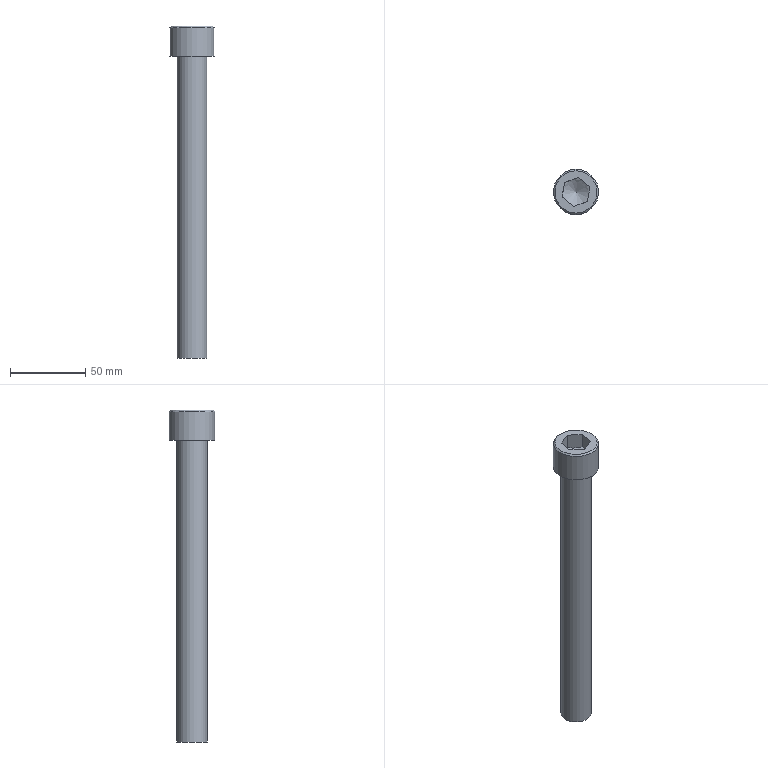Part | NX | features solid 2 | 1 solid | 13 faces | box 30 x 30 x 220 mm | volume 73865 mm3 | plane 9 | cone 2 | cylinder 2 | commonest cylinder face diameters 20 x1 30 x1
STEP:
#1=CARTESIAN_POINT('',(-425.,274.,-24.));
#2=VERTEX_POINT('',#1);
#3=CARTESIAN_POINT('',(-425.,260.,-24.));
#4=DIRECTION('',(0.,0.,-1.));
#5=DIRECTION('',(0.,1.,0.));
#6=AXIS2_PLACEMENT_3D('',#3,#4,#5);
#7=CIRCLE('',#6,14.);
#8=EDGE_CURVE('',#2,#2,#7,.T.);
#9=ORIENTED_EDGE('',*,*,#8,.F.);
#10=EDGE_LOOP('',(#9));
#11=FACE_BOUND('',#10,.T.);
#12=CARTESIAN_POINT('',(-434.201,256.582,-24.));
#13=VERTEX_POINT('',#12);
#14=CARTESIAN_POINT('',(-426.641,250.323,-24.));
#15=VERTEX_POINT('',#14);
#16=CARTESIAN_POINT('',(-430.421,253.453,-24.));
#17=DIRECTION('',(0.7703,-0.6377,0.));
#18=VECTOR('',#17,1000.);
#19=LINE('',#16,#18);
#20=EDGE_CURVE('',#13,#15,#19,.T.);
#21=ORIENTED_EDGE('',*,*,#20,.F.);
#22=CARTESIAN_POINT('',(-432.56,266.259,-24.));
#23=VERTEX_POINT('',#22);
#24=CARTESIAN_POINT('',(-433.38,261.421,-24.));
#25=DIRECTION('',(-0.1672,-0.9859,0.));
#26=VECTOR('',#25,1000.);
#27=LINE('',#24,#26);
#28=EDGE_CURVE('',#23,#13,#27,.T.);
#29=ORIENTED_EDGE('',*,*,#28,.F.);
#30=CARTESIAN_POINT('',(-423.359,269.677,-24.));
#31=VERTEX_POINT('',#30);
#32=CARTESIAN_POINT('',(-427.96,267.968,-24.));
#33=DIRECTION('',(-0.9374,-0.3482,0.));
#34=VECTOR('',#33,1000.);
#35=LINE('',#32,#34);
#36=EDGE_CURVE('',#31,#23,#35,.T.);
#37=ORIENTED_EDGE('',*,*,#36,.F.);
#38=CARTESIAN_POINT('',(-415.799,263.418,-24.));
#39=VERTEX_POINT('',#38);
#40=CARTESIAN_POINT('',(-419.579,266.547,-24.));
#41=DIRECTION('',(-0.7703,0.6377,0.));
#42=VECTOR('',#41,1000.);
#43=LINE('',#40,#42);
#44=EDGE_CURVE('',#39,#31,#43,.T.);
#45=ORIENTED_EDGE('',*,*,#44,.F.);
#46=CARTESIAN_POINT('',(-417.44,253.741,-24.));
#47=VERTEX_POINT('',#46);
#48=CARTESIAN_POINT('',(-416.62,258.579,-24.));
#49=DIRECTION('',(0.1672,0.9859,0.));
#50=VECTOR('',#49,1000.);
#51=LINE('',#48,#50);
#52=EDGE_CURVE('',#47,#39,#51,.T.);
#53=ORIENTED_EDGE('',*,*,#52,.F.);
#54=CARTESIAN_POINT('',(-422.04,252.032,-24.));
#55=DIRECTION('',(0.9374,0.3482,0.));
#56=VECTOR('',#55,1000.);
#57=LINE('',#54,#56);
#58=EDGE_CURVE('',#15,#47,#57,.T.);
#59=ORIENTED_EDGE('',*,*,#58,.F.);
#60=EDGE_LOOP('',(#21,#29,#37,#45,#53,#59));
#61=FACE_BOUND('',#60,.T.);
#62=CARTESIAN_POINT('',(-425.,260.,-24.));
#63=DIRECTION('',(0.,0.,-1.));
#64=DIRECTION('',(0.,1.,0.));
#65=AXIS2_PLACEMENT_3D('',#62,#63,#64);
#66=PLANE('',#65);
#67=ADVANCED_FACE('',(#11,#61),#66,.F.);
#68=CARTESIAN_POINT('',(-425.,250.,-244.));
#69=VERTEX_POINT('',#68);
#70=CARTESIAN_POINT('',(-425.,260.,-244.));
#71=DIRECTION('',(0.,0.,1.));
#72=DIRECTION('',(0.,-1.,0.));
#73=AXIS2_PLACEMENT_3D('',#70,#71,#72);
#74=CIRCLE('',#73,10.);
#75=EDGE_CURVE('',#69,#69,#74,.F.);
#76=ORIENTED_EDGE('',*,*,#75,.T.);
#77=EDGE_LOOP('',(#76));
#78=FACE_BOUND('',#77,.T.);
#79=CARTESIAN_POINT('',(-425.,269.,-244.));
#80=DIRECTION('',(0.,0.,1.));
#81=DIRECTION('',(0.,-1.,0.));
#82=AXIS2_PLACEMENT_3D('',#79,#80,#81);
#83=PLANE('',#82);
#84=ADVANCED_FACE('',(#78),#83,.F.);
#85=CARTESIAN_POINT('',(-425.,275.,-25.));
#86=VERTEX_POINT('',#85);
#87=CARTESIAN_POINT('',(-425.,260.,-25.));
#88=DIRECTION('',(0.,0.,-1.));
#89=DIRECTION('',(0.,1.,0.));
#90=AXIS2_PLACEMENT_3D('',#87,#88,#89);
#91=CIRCLE('',#90,15.);
#92=EDGE_CURVE('',#86,#86,#91,.T.);
#93=ORIENTED_EDGE('',*,*,#92,.F.);
#94=EDGE_LOOP('',(#93));
#95=FACE_BOUND('',#94,.T.);
#96=ORIENTED_EDGE('',*,*,#8,.T.);
#97=EDGE_LOOP('',(#96));
#98=FACE_BOUND('',#97,.T.);
#99=CARTESIAN_POINT('',(-425.,260.,-24.));
#100=DIRECTION('',(0.,0.,-1.));
#101=DIRECTION('',(0.,1.,0.));
#102=AXIS2_PLACEMENT_3D('',#99,#100,#101);
#103=CONICAL_SURFACE('',#102,14.,0.7854);
#104=ADVANCED_FACE('',(#95,#98),#103,.T.);
#105=CARTESIAN_POINT('',(-425.,275.,-44.));
#106=VERTEX_POINT('',#105);
#107=CARTESIAN_POINT('',(-425.,260.,-44.));
#108=DIRECTION('',(0.,0.,-1.));
#109=DIRECTION('',(0.,1.,0.));
#110=AXIS2_PLACEMENT_3D('',#107,#108,#109);
#111=CIRCLE('',#110,15.);
#112=EDGE_CURVE('',#106,#106,#111,.T.);
#113=ORIENTED_EDGE('',*,*,#112,.F.);
#114=EDGE_LOOP('',(#113));
#115=FACE_BOUND('',#114,.T.);
#116=ORIENTED_EDGE('',*,*,#92,.T.);
#117=EDGE_LOOP('',(#116));
#118=FACE_BOUND('',#117,.T.);
#119=CARTESIAN_POINT('',(-425.,260.,-24.));
#120=DIRECTION('',(0.,0.,-1.));
#121=DIRECTION('',(0.,1.,0.));
#122=AXIS2_PLACEMENT_3D('',#119,#120,#121);
#123=CYLINDRICAL_SURFACE('',#122,15.);
#124=ADVANCED_FACE('',(#115,#118),#123,.T.);
#125=CARTESIAN_POINT('',(-425.,270.,-44.));
#126=VERTEX_POINT('',#125);
#127=CARTESIAN_POINT('',(-425.,260.,-44.));
#128=DIRECTION('',(0.,0.,-1.));
#129=DIRECTION('',(0.,1.,0.));
#130=AXIS2_PLACEMENT_3D('',#127,#128,#129);
#131=CIRCLE('',#130,10.);
#132=EDGE_CURVE('',#126,#126,#131,.T.);
#133=ORIENTED_EDGE('',*,*,#132,.F.);
#134=EDGE_LOOP('',(#133));
#135=FACE_BOUND('',#134,.T.);
#136=ORIENTED_EDGE('',*,*,#112,.T.);
#137=EDGE_LOOP('',(#136));
#138=FACE_BOUND('',#137,.T.);
#139=CARTESIAN_POINT('',(-425.,275.,-44.));
#140=DIRECTION('',(0.,0.,1.));
#141=DIRECTION('',(0.,-1.,0.));
#142=AXIS2_PLACEMENT_3D('',#139,#140,#141);
#143=PLANE('',#142);
#144=ADVANCED_FACE('',(#135,#138),#143,.F.);
#145=ORIENTED_EDGE('',*,*,#75,.F.);
#146=EDGE_LOOP('',(#145));
#147=FACE_BOUND('',#146,.T.);
#148=ORIENTED_EDGE('',*,*,#132,.T.);
#149=EDGE_LOOP('',(#148));
#150=FACE_BOUND('',#149,.T.);
#151=CARTESIAN_POINT('',(-425.,260.,-24.));
#152=DIRECTION('',(0.,0.,-1.));
#153=DIRECTION('',(0.,1.,0.));
#154=AXIS2_PLACEMENT_3D('',#151,#152,#153);
#155=CYLINDRICAL_SURFACE('',#154,10.);
#156=ADVANCED_FACE('',(#147,#150),#155,.T.);
#157=ORIENTED_EDGE('',*,*,#20,.T.);
#158=CARTESIAN_POINT('',(-426.641,250.323,-34.));
#159=VERTEX_POINT('',#158);
#160=CARTESIAN_POINT('',(-426.641,250.323,-44.));
#161=DIRECTION('',(0.,0.,1.));
#162=VECTOR('',#161,1000.);
#163=LINE('',#160,#162);
#164=EDGE_CURVE('',#159,#15,#163,.T.);
#165=ORIENTED_EDGE('',*,*,#164,.F.);
#166=CARTESIAN_POINT('',(-434.201,256.582,-34.));
#167=VERTEX_POINT('',#166);
#168=CARTESIAN_POINT('',(-434.201,256.582,-34.));
#169=CARTESIAN_POINT('',(-432.966,255.56,-34.463));
#170=CARTESIAN_POINT('',(-430.434,253.464,-35.055));
#171=CARTESIAN_POINT('',(-427.877,251.346,-34.463));
#172=CARTESIAN_POINT('',(-426.641,250.323,-34.));
#173=B_SPLINE_CURVE_WITH_KNOTS('',3,(#168,#169,#170,#171,#172),.UNSPECIFIED.,.F.,.F.,(4,1,4),(0.,0.004956,0.009913),.UNSPECIFIED.);
#174=EDGE_CURVE('',#167,#159,#173,.T.);
#175=ORIENTED_EDGE('',*,*,#174,.F.);
#176=CARTESIAN_POINT('',(-434.201,256.582,-44.));
#177=DIRECTION('',(0.,0.,1.));
#178=VECTOR('',#177,1000.);
#179=LINE('',#176,#178);
#180=EDGE_CURVE('',#167,#13,#179,.T.);
#181=ORIENTED_EDGE('',*,*,#180,.T.);
#182=EDGE_LOOP('',(#157,#165,#175,#181));
#183=FACE_BOUND('',#182,.T.);
#184=CARTESIAN_POINT('',(-426.641,250.323,-44.));
#185=DIRECTION('',(0.6377,0.7703,0.));
#186=DIRECTION('',(-0.7703,0.6377,0.));
#187=AXIS2_PLACEMENT_3D('',#184,#185,#186);
#188=PLANE('',#187);
#189=ADVANCED_FACE('',(#183),#188,.T.);
#190=ORIENTED_EDGE('',*,*,#28,.T.);
#191=ORIENTED_EDGE('',*,*,#180,.F.);
#192=CARTESIAN_POINT('',(-432.56,266.259,-34.));
#193=VERTEX_POINT('',#192);
#194=CARTESIAN_POINT('',(-432.56,266.259,-34.));
#195=CARTESIAN_POINT('',(-432.828,264.679,-34.463));
#196=CARTESIAN_POINT('',(-433.377,261.438,-35.055));
#197=CARTESIAN_POINT('',(-433.933,258.164,-34.463));
#198=CARTESIAN_POINT('',(-434.201,256.582,-34.));
#199=B_SPLINE_CURVE_WITH_KNOTS('',3,(#194,#195,#196,#197,#198),.UNSPECIFIED.,.F.,.F.,(4,1,4),(0.,0.004956,0.009913),.UNSPECIFIED.);
#200=EDGE_CURVE('',#193,#167,#199,.T.);
#201=ORIENTED_EDGE('',*,*,#200,.F.);
#202=CARTESIAN_POINT('',(-432.56,266.259,-44.));
#203=DIRECTION('',(0.,0.,1.));
#204=VECTOR('',#203,1000.);
#205=LINE('',#202,#204);
#206=EDGE_CURVE('',#193,#23,#205,.T.);
#207=ORIENTED_EDGE('',*,*,#206,.T.);
#208=EDGE_LOOP('',(#190,#191,#201,#207));
#209=FACE_BOUND('',#208,.T.);
#210=CARTESIAN_POINT('',(-434.201,256.582,-44.));
#211=DIRECTION('',(0.9859,-0.1672,0.));
#212=DIRECTION('',(0.1672,0.9859,0.));
#213=AXIS2_PLACEMENT_3D('',#210,#211,#212);
#214=PLANE('',#213);
#215=ADVANCED_FACE('',(#209),#214,.T.);
#216=ORIENTED_EDGE('',*,*,#36,.T.);
#217=ORIENTED_EDGE('',*,*,#206,.F.);
#218=CARTESIAN_POINT('',(-423.359,269.677,-34.));
#219=VERTEX_POINT('',#218);
#220=CARTESIAN_POINT('',(-423.359,269.677,-34.));
#221=CARTESIAN_POINT('',(-424.862,269.119,-34.463));
#222=CARTESIAN_POINT('',(-427.943,267.974,-35.055));
#223=CARTESIAN_POINT('',(-431.056,266.818,-34.463));
#224=CARTESIAN_POINT('',(-432.56,266.259,-34.));
#225=B_SPLINE_CURVE_WITH_KNOTS('',3,(#220,#221,#222,#223,#224),.UNSPECIFIED.,.F.,.F.,(4,1,4),(0.,0.004956,0.009913),.UNSPECIFIED.);
#226=EDGE_CURVE('',#219,#193,#225,.T.);
#227=ORIENTED_EDGE('',*,*,#226,.F.);
#228=CARTESIAN_POINT('',(-423.359,269.677,-44.));
#229=DIRECTION('',(0.,0.,1.));
#230=VECTOR('',#229,1000.);
#231=LINE('',#228,#230);
#232=EDGE_CURVE('',#219,#31,#231,.T.);
#233=ORIENTED_EDGE('',*,*,#232,.T.);
#234=EDGE_LOOP('',(#216,#217,#227,#233));
#235=FACE_BOUND('',#234,.T.);
#236=CARTESIAN_POINT('',(-432.56,266.259,-44.));
#237=DIRECTION('',(0.3482,-0.9374,0.));
#238=DIRECTION('',(0.9374,0.3482,0.));
#239=AXIS2_PLACEMENT_3D('',#236,#237,#238);
#240=PLANE('',#239);
#241=ADVANCED_FACE('',(#235),#240,.T.);
#242=ORIENTED_EDGE('',*,*,#44,.T.);
#243=ORIENTED_EDGE('',*,*,#232,.F.);
#244=CARTESIAN_POINT('',(-415.799,263.418,-34.));
#245=VERTEX_POINT('',#244);
#246=CARTESIAN_POINT('',(-415.799,263.418,-34.));
#247=CARTESIAN_POINT('',(-417.034,264.44,-34.463));
#248=CARTESIAN_POINT('',(-419.566,266.536,-35.055));
#249=CARTESIAN_POINT('',(-422.123,268.654,-34.463));
#250=CARTESIAN_POINT('',(-423.359,269.677,-34.));
#251=B_SPLINE_CURVE_WITH_KNOTS('',3,(#246,#247,#248,#249,#250),.UNSPECIFIED.,.F.,.F.,(4,1,4),(0.,0.004956,0.009913),.UNSPECIFIED.);
#252=EDGE_CURVE('',#245,#219,#251,.T.);
#253=ORIENTED_EDGE('',*,*,#252,.F.);
#254=CARTESIAN_POINT('',(-415.799,263.418,-44.));
#255=DIRECTION('',(0.,0.,1.));
#256=VECTOR('',#255,1000.);
#257=LINE('',#254,#256);
#258=EDGE_CURVE('',#245,#39,#257,.T.);
#259=ORIENTED_EDGE('',*,*,#258,.T.);
#260=EDGE_LOOP('',(#242,#243,#253,#259));
#261=FACE_BOUND('',#260,.T.);
#262=CARTESIAN_POINT('',(-423.359,269.677,-44.));
#263=DIRECTION('',(-0.6377,-0.7703,0.));
#264=DIRECTION('',(0.7703,-0.6377,0.));
#265=AXIS2_PLACEMENT_3D('',#262,#263,#264);
#266=PLANE('',#265);
#267=ADVANCED_FACE('',(#261),#266,.T.);
#268=ORIENTED_EDGE('',*,*,#52,.T.);
#269=ORIENTED_EDGE('',*,*,#258,.F.);
#270=CARTESIAN_POINT('',(-417.44,253.741,-34.));
#271=VERTEX_POINT('',#270);
#272=CARTESIAN_POINT('',(-417.44,253.741,-34.));
#273=CARTESIAN_POINT('',(-417.172,255.321,-34.463));
#274=CARTESIAN_POINT('',(-416.623,258.562,-35.055));
#275=CARTESIAN_POINT('',(-416.067,261.836,-34.463));
#276=CARTESIAN_POINT('',(-415.799,263.418,-34.));
#277=B_SPLINE_CURVE_WITH_KNOTS('',3,(#272,#273,#274,#275,#276),.UNSPECIFIED.,.F.,.F.,(4,1,4),(0.,0.004956,0.009913),.UNSPECIFIED.);
#278=EDGE_CURVE('',#271,#245,#277,.T.);
#279=ORIENTED_EDGE('',*,*,#278,.F.);
#280=CARTESIAN_POINT('',(-417.44,253.741,-44.));
#281=DIRECTION('',(0.,0.,1.));
#282=VECTOR('',#281,1000.);
#283=LINE('',#280,#282);
#284=EDGE_CURVE('',#271,#47,#283,.T.);
#285=ORIENTED_EDGE('',*,*,#284,.T.);
#286=EDGE_LOOP('',(#268,#269,#279,#285));
#287=FACE_BOUND('',#286,.T.);
#288=CARTESIAN_POINT('',(-415.799,263.418,-44.));
#289=DIRECTION('',(-0.9859,0.1672,0.));
#290=DIRECTION('',(-0.1672,-0.9859,0.));
#291=AXIS2_PLACEMENT_3D('',#288,#289,#290);
#292=PLANE('',#291);
#293=ADVANCED_FACE('',(#287),#292,.T.);
#294=ORIENTED_EDGE('',*,*,#58,.T.);
#295=ORIENTED_EDGE('',*,*,#284,.F.);
#296=CARTESIAN_POINT('',(-426.641,250.323,-34.));
#297=CARTESIAN_POINT('',(-425.138,250.881,-34.463));
#298=CARTESIAN_POINT('',(-422.057,252.026,-35.055));
#299=CARTESIAN_POINT('',(-418.944,253.182,-34.463));
#300=CARTESIAN_POINT('',(-417.44,253.741,-34.));
#301=B_SPLINE_CURVE_WITH_KNOTS('',3,(#296,#297,#298,#299,#300),.UNSPECIFIED.,.F.,.F.,(4,1,4),(0.,0.004956,0.009913),.UNSPECIFIED.);
#302=EDGE_CURVE('',#159,#271,#301,.T.);
#303=ORIENTED_EDGE('',*,*,#302,.F.);
#304=ORIENTED_EDGE('',*,*,#164,.T.);
#305=EDGE_LOOP('',(#294,#295,#303,#304));
#306=FACE_BOUND('',#305,.T.);
#307=CARTESIAN_POINT('',(-417.44,253.741,-44.));
#308=DIRECTION('',(-0.3482,0.9374,0.));
#309=DIRECTION('',(-0.9374,-0.3482,0.));
#310=AXIS2_PLACEMENT_3D('',#307,#308,#309);
#311=PLANE('',#310);
#312=ADVANCED_FACE('',(#306),#311,.T.);
#313=CARTESIAN_POINT('',(-425.,260.,-39.667));
#314=VERTEX_POINT('',#313);
#315=VERTEX_LOOP('',#314);
#316=FACE_BOUND('',#315,.T.);
#317=ORIENTED_EDGE('',*,*,#174,.T.);
#318=ORIENTED_EDGE('',*,*,#302,.T.);
#319=ORIENTED_EDGE('',*,*,#278,.T.);
#320=ORIENTED_EDGE('',*,*,#252,.T.);
#321=ORIENTED_EDGE('',*,*,#226,.T.);
#322=ORIENTED_EDGE('',*,*,#200,.T.);
#323=EDGE_LOOP('',(#317,#318,#319,#320,#321,#322));
#324=FACE_BOUND('',#323,.T.);
#325=CARTESIAN_POINT('',(-425.,260.,-31.006));
#326=DIRECTION('',(0.,0.,1.));
#327=DIRECTION('',(1.,0.,0.));
#328=AXIS2_PLACEMENT_3D('',#325,#326,#327);
#329=CONICAL_SURFACE('',#328,15.,1.047);
#330=ADVANCED_FACE('',(#316,#324),#329,.F.);
#331=CLOSED_SHELL('',(#67,#84,#104,#124,#144,#156,#189,#215,#241,#267,#293,#312,#330));
#332=MANIFOLD_SOLID_BREP('',#331);
#333=(LENGTH_UNIT()NAMED_UNIT(*)SI_UNIT(.MILLI.,.METRE.));
#334=UNCERTAINTY_MEASURE_WITH_UNIT(LENGTH_MEASURE(0.0508),#333,'','');
#335=(NAMED_UNIT(*)PLANE_ANGLE_UNIT()SI_UNIT($,.RADIAN.));
#336=(NAMED_UNIT(*)SI_UNIT($,.STERADIAN.)SOLID_ANGLE_UNIT());
#337=(GEOMETRIC_REPRESENTATION_CONTEXT(3)GLOBAL_UNCERTAINTY_ASSIGNED_CONTEXT((#334))GLOBAL_UNIT_ASSIGNED_CONTEXT((#333,#335,#336))REPRESENTATION_CONTEXT('',''));
#338=ADVANCED_BREP_SHAPE_REPRESENTATION('',(#332),#337);